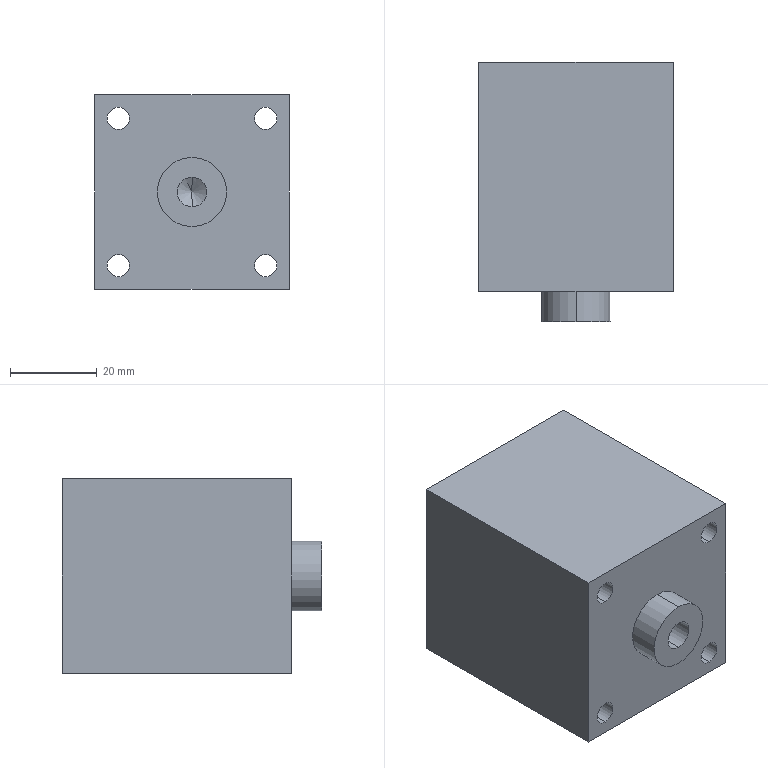Part | STEP file | 1 solid | 33 faces | box 45 x 60 x 45 mm | volume 101884 mm3 | cylinder 20 | plane 11 | cone 2 | commonest cylinder face diameters 5.2 x8 10 x8 6.8 x2 16 x2